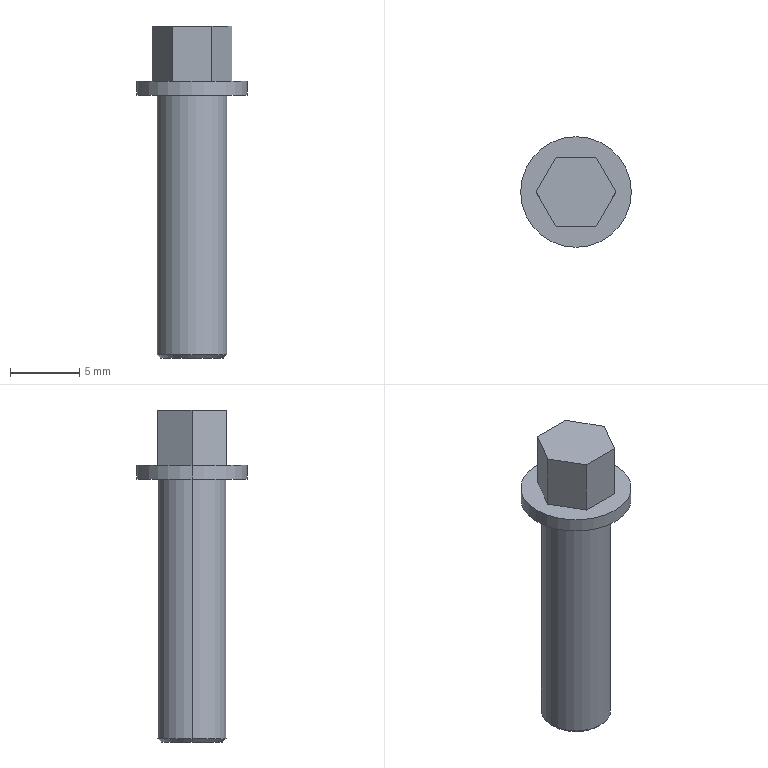Part | SolidWorks | features BaseBody 1 | 1 solid | 16 faces | box 8 x 8 x 24 mm | volume 509.458 mm3 | plane 10 | cylinder 4 | cone 2 | commonest cylinder face diameters 5 x2 8 x2
STEP:
#1=CARTESIAN_POINT('',(2.25,0.,-19.));
#2=VERTEX_POINT('',#1);
#3=CARTESIAN_POINT('',(-2.25,0.,-19.));
#4=VERTEX_POINT('',#3);
#5=CARTESIAN_POINT('',(0.,0.,-19.));
#6=DIRECTION('',(0.,0.,1.));
#7=DIRECTION('',(1.,0.,0.));
#8=AXIS2_PLACEMENT_3D('',#5,#6,#7);
#9=CIRCLE('',#8,2.25);
#10=EDGE_CURVE('',#2,#4,#9,.T.);
#11=ORIENTED_EDGE('',*,*,#10,.T.);
#12=CARTESIAN_POINT('',(-2.5,0.,-18.75));
#13=VERTEX_POINT('',#12);
#14=CARTESIAN_POINT('',(-2.375,0.,-18.875));
#15=DIRECTION('',(-0.7071,0.,0.7071));
#16=VECTOR('',#15,1000.);
#17=LINE('',#14,#16);
#18=EDGE_CURVE('',#4,#13,#17,.T.);
#19=ORIENTED_EDGE('',*,*,#18,.T.);
#20=CARTESIAN_POINT('',(2.5,0.,-18.75));
#21=VERTEX_POINT('',#20);
#22=CARTESIAN_POINT('',(0.,0.,-18.75));
#23=DIRECTION('',(0.,0.,-1.));
#24=DIRECTION('',(1.,0.,0.));
#25=AXIS2_PLACEMENT_3D('',#22,#23,#24);
#26=CIRCLE('',#25,2.5);
#27=EDGE_CURVE('',#13,#21,#26,.T.);
#28=ORIENTED_EDGE('',*,*,#27,.T.);
#29=CARTESIAN_POINT('',(2.375,0.,-18.875));
#30=DIRECTION('',(0.7071,0.,0.7071));
#31=VECTOR('',#30,1000.);
#32=LINE('',#29,#31);
#33=EDGE_CURVE('',#2,#21,#32,.T.);
#34=ORIENTED_EDGE('',*,*,#33,.F.);
#35=EDGE_LOOP('',(#11,#19,#28,#34));
#36=FACE_OUTER_BOUND('',#35,.T.);
#37=CARTESIAN_POINT('',(0.,0.,-18.875));
#38=DIRECTION('',(0.,0.,1.));
#39=DIRECTION('',(1.,0.,0.));
#40=AXIS2_PLACEMENT_3D('',#37,#38,#39);
#41=CONICAL_SURFACE('',#40,2.375,0.7854);
#42=ADVANCED_FACE('',(#36),#41,.T.);
#43=ORIENTED_EDGE('',*,*,#27,.F.);
#44=CARTESIAN_POINT('',(-2.5,0.,0.));
#45=VERTEX_POINT('',#44);
#46=CARTESIAN_POINT('',(-2.5,0.,0.));
#47=DIRECTION('',(0.,0.,1.));
#48=VECTOR('',#47,1000.);
#49=LINE('',#46,#48);
#50=EDGE_CURVE('',#13,#45,#49,.T.);
#51=ORIENTED_EDGE('',*,*,#50,.T.);
#52=CARTESIAN_POINT('',(2.5,0.,0.));
#53=VERTEX_POINT('',#52);
#54=CARTESIAN_POINT('',(0.,0.,0.));
#55=DIRECTION('',(0.,0.,1.));
#56=DIRECTION('',(1.,0.,0.));
#57=AXIS2_PLACEMENT_3D('',#54,#55,#56);
#58=CIRCLE('',#57,2.5);
#59=EDGE_CURVE('',#53,#45,#58,.T.);
#60=ORIENTED_EDGE('',*,*,#59,.F.);
#61=CARTESIAN_POINT('',(2.5,0.,0.));
#62=DIRECTION('',(0.,0.,1.));
#63=VECTOR('',#62,1000.);
#64=LINE('',#61,#63);
#65=EDGE_CURVE('',#21,#53,#64,.T.);
#66=ORIENTED_EDGE('',*,*,#65,.F.);
#67=EDGE_LOOP('',(#43,#51,#60,#66));
#68=FACE_OUTER_BOUND('',#67,.T.);
#69=CARTESIAN_POINT('',(0.,0.,0.));
#70=DIRECTION('',(0.,0.,1.));
#71=DIRECTION('',(1.,0.,0.));
#72=AXIS2_PLACEMENT_3D('',#69,#70,#71);
#73=CYLINDRICAL_SURFACE('',#72,2.5);
#74=ADVANCED_FACE('',(#68),#73,.T.);
#75=CARTESIAN_POINT('',(4.,0.,1.));
#76=VERTEX_POINT('',#75);
#77=CARTESIAN_POINT('',(-4.,0.,1.));
#78=VERTEX_POINT('',#77);
#79=CARTESIAN_POINT('',(0.,0.,1.));
#80=DIRECTION('',(0.,0.,1.));
#81=DIRECTION('',(-1.,0.,0.));
#82=AXIS2_PLACEMENT_3D('',#79,#80,#81);
#83=CIRCLE('',#82,4.);
#84=EDGE_CURVE('',#76,#78,#83,.T.);
#85=ORIENTED_EDGE('',*,*,#84,.F.);
#86=CARTESIAN_POINT('',(4.,0.,0.));
#87=VERTEX_POINT('',#86);
#88=CARTESIAN_POINT('',(4.,0.,0.));
#89=DIRECTION('',(0.,0.,-1.));
#90=VECTOR('',#89,1000.);
#91=LINE('',#88,#90);
#92=EDGE_CURVE('',#76,#87,#91,.T.);
#93=ORIENTED_EDGE('',*,*,#92,.T.);
#94=CARTESIAN_POINT('',(-4.,0.,0.));
#95=VERTEX_POINT('',#94);
#96=CARTESIAN_POINT('',(0.,0.,0.));
#97=DIRECTION('',(0.,0.,-1.));
#98=DIRECTION('',(-1.,0.,0.));
#99=AXIS2_PLACEMENT_3D('',#96,#97,#98);
#100=CIRCLE('',#99,4.);
#101=EDGE_CURVE('',#95,#87,#100,.T.);
#102=ORIENTED_EDGE('',*,*,#101,.F.);
#103=CARTESIAN_POINT('',(-4.,0.,0.));
#104=DIRECTION('',(0.,0.,-1.));
#105=VECTOR('',#104,1000.);
#106=LINE('',#103,#105);
#107=EDGE_CURVE('',#78,#95,#106,.T.);
#108=ORIENTED_EDGE('',*,*,#107,.F.);
#109=EDGE_LOOP('',(#85,#93,#102,#108));
#110=FACE_OUTER_BOUND('',#109,.T.);
#111=CARTESIAN_POINT('',(0.,0.,0.));
#112=DIRECTION('',(0.,0.,-1.));
#113=DIRECTION('',(-1.,0.,0.));
#114=AXIS2_PLACEMENT_3D('',#111,#112,#113);
#115=CYLINDRICAL_SURFACE('',#114,4.);
#116=ADVANCED_FACE('',(#110),#115,.T.);
#117=ORIENTED_EDGE('',*,*,#10,.F.);
#118=CARTESIAN_POINT('',(0.,0.,-19.));
#119=DIRECTION('',(0.,0.,1.));
#120=DIRECTION('',(1.,0.,0.));
#121=AXIS2_PLACEMENT_3D('',#118,#119,#120);
#122=CIRCLE('',#121,2.25);
#123=EDGE_CURVE('',#4,#2,#122,.T.);
#124=ORIENTED_EDGE('',*,*,#123,.F.);
#125=EDGE_LOOP('',(#117,#124));
#126=FACE_OUTER_BOUND('',#125,.T.);
#127=CARTESIAN_POINT('',(0.,0.,-19.));
#128=DIRECTION('',(0.,0.,1.));
#129=DIRECTION('',(1.,0.,0.));
#130=AXIS2_PLACEMENT_3D('',#127,#128,#129);
#131=PLANE('',#130);
#132=ADVANCED_FACE('',(#126),#131,.F.);
#133=CARTESIAN_POINT('',(-1.443,-2.5,1.));
#134=VERTEX_POINT('',#133);
#135=CARTESIAN_POINT('',(-2.887,0.,1.));
#136=VERTEX_POINT('',#135);
#137=CARTESIAN_POINT('',(-2.526,-0.625,1.));
#138=DIRECTION('',(-0.5,0.866,0.));
#139=VECTOR('',#138,1000.);
#140=LINE('',#137,#139);
#141=EDGE_CURVE('',#134,#136,#140,.T.);
#142=ORIENTED_EDGE('',*,*,#141,.F.);
#143=CARTESIAN_POINT('',(-1.443,-2.5,5.));
#144=VERTEX_POINT('',#143);
#145=CARTESIAN_POINT('',(-1.443,-2.5,1.));
#146=DIRECTION('',(0.,0.,1.));
#147=VECTOR('',#146,1000.);
#148=LINE('',#145,#147);
#149=EDGE_CURVE('',#134,#144,#148,.T.);
#150=ORIENTED_EDGE('',*,*,#149,.T.);
#151=CARTESIAN_POINT('',(-2.887,0.,5.));
#152=VERTEX_POINT('',#151);
#153=CARTESIAN_POINT('',(-1.443,-2.5,5.));
#154=DIRECTION('',(0.5,-0.866,0.));
#155=VECTOR('',#154,1000.);
#156=LINE('',#153,#155);
#157=EDGE_CURVE('',#152,#144,#156,.T.);
#158=ORIENTED_EDGE('',*,*,#157,.F.);
#159=CARTESIAN_POINT('',(-2.887,0.,1.));
#160=DIRECTION('',(0.,0.,1.));
#161=VECTOR('',#160,1000.);
#162=LINE('',#159,#161);
#163=EDGE_CURVE('',#136,#152,#162,.T.);
#164=ORIENTED_EDGE('',*,*,#163,.F.);
#165=EDGE_LOOP('',(#142,#150,#158,#164));
#166=FACE_OUTER_BOUND('',#165,.T.);
#167=CARTESIAN_POINT('',(-2.887,0.,1.));
#168=DIRECTION('',(-0.866,-0.5,0.));
#169=DIRECTION('',(-0.5,0.866,0.));
#170=AXIS2_PLACEMENT_3D('',#167,#168,#169);
#171=PLANE('',#170);
#172=ADVANCED_FACE('',(#166),#171,.T.);
#173=CARTESIAN_POINT('',(-1.443,2.5,1.));
#174=VERTEX_POINT('',#173);
#175=CARTESIAN_POINT('',(-1.804,1.875,1.));
#176=DIRECTION('',(0.5,0.866,0.));
#177=VECTOR('',#176,1000.);
#178=LINE('',#175,#177);
#179=EDGE_CURVE('',#136,#174,#178,.T.);
#180=ORIENTED_EDGE('',*,*,#179,.F.);
#181=ORIENTED_EDGE('',*,*,#163,.T.);
#182=CARTESIAN_POINT('',(-1.443,2.5,5.));
#183=VERTEX_POINT('',#182);
#184=CARTESIAN_POINT('',(-2.887,0.,5.));
#185=DIRECTION('',(-0.5,-0.866,0.));
#186=VECTOR('',#185,1000.);
#187=LINE('',#184,#186);
#188=EDGE_CURVE('',#183,#152,#187,.T.);
#189=ORIENTED_EDGE('',*,*,#188,.F.);
#190=CARTESIAN_POINT('',(-1.443,2.5,1.));
#191=DIRECTION('',(0.,0.,1.));
#192=VECTOR('',#191,1000.);
#193=LINE('',#190,#192);
#194=EDGE_CURVE('',#174,#183,#193,.T.);
#195=ORIENTED_EDGE('',*,*,#194,.F.);
#196=EDGE_LOOP('',(#180,#181,#189,#195));
#197=FACE_OUTER_BOUND('',#196,.T.);
#198=CARTESIAN_POINT('',(-1.443,2.5,1.));
#199=DIRECTION('',(-0.866,0.5,0.));
#200=DIRECTION('',(0.,0.,1.));
#201=AXIS2_PLACEMENT_3D('',#198,#199,#200);
#202=PLANE('',#201);
#203=ADVANCED_FACE('',(#197),#202,.T.);
#204=CARTESIAN_POINT('',(1.443,2.5,1.));
#205=VERTEX_POINT('',#204);
#206=CARTESIAN_POINT('',(0.7217,2.5,1.));
#207=DIRECTION('',(1.,0.,0.));
#208=VECTOR('',#207,1000.);
#209=LINE('',#206,#208);
#210=EDGE_CURVE('',#174,#205,#209,.T.);
#211=ORIENTED_EDGE('',*,*,#210,.F.);
#212=ORIENTED_EDGE('',*,*,#194,.T.);
#213=CARTESIAN_POINT('',(1.443,2.5,5.));
#214=VERTEX_POINT('',#213);
#215=CARTESIAN_POINT('',(-1.443,2.5,5.));
#216=DIRECTION('',(-1.,0.,0.));
#217=VECTOR('',#216,1000.);
#218=LINE('',#215,#217);
#219=EDGE_CURVE('',#214,#183,#218,.T.);
#220=ORIENTED_EDGE('',*,*,#219,.F.);
#221=CARTESIAN_POINT('',(1.443,2.5,1.));
#222=DIRECTION('',(0.,0.,1.));
#223=VECTOR('',#222,1000.);
#224=LINE('',#221,#223);
#225=EDGE_CURVE('',#205,#214,#224,.T.);
#226=ORIENTED_EDGE('',*,*,#225,.F.);
#227=EDGE_LOOP('',(#211,#212,#220,#226));
#228=FACE_OUTER_BOUND('',#227,.T.);
#229=CARTESIAN_POINT('',(1.443,2.5,1.));
#230=DIRECTION('',(0.,1.,0.));
#231=DIRECTION('',(1.,0.,0.));
#232=AXIS2_PLACEMENT_3D('',#229,#230,#231);
#233=PLANE('',#232);
#234=ADVANCED_FACE('',(#228),#233,.T.);
#235=CARTESIAN_POINT('',(2.887,0.,1.));
#236=VERTEX_POINT('',#235);
#237=CARTESIAN_POINT('',(2.526,0.625,1.));
#238=DIRECTION('',(0.5,-0.866,0.));
#239=VECTOR('',#238,1000.);
#240=LINE('',#237,#239);
#241=EDGE_CURVE('',#205,#236,#240,.T.);
#242=ORIENTED_EDGE('',*,*,#241,.F.);
#243=ORIENTED_EDGE('',*,*,#225,.T.);
#244=CARTESIAN_POINT('',(2.887,0.,5.));
#245=VERTEX_POINT('',#244);
#246=CARTESIAN_POINT('',(1.443,2.5,5.));
#247=DIRECTION('',(-0.5,0.866,0.));
#248=VECTOR('',#247,1000.);
#249=LINE('',#246,#248);
#250=EDGE_CURVE('',#245,#214,#249,.T.);
#251=ORIENTED_EDGE('',*,*,#250,.F.);
#252=CARTESIAN_POINT('',(2.887,0.,1.));
#253=DIRECTION('',(0.,0.,1.));
#254=VECTOR('',#253,1000.);
#255=LINE('',#252,#254);
#256=EDGE_CURVE('',#236,#245,#255,.T.);
#257=ORIENTED_EDGE('',*,*,#256,.F.);
#258=EDGE_LOOP('',(#242,#243,#251,#257));
#259=FACE_OUTER_BOUND('',#258,.T.);
#260=CARTESIAN_POINT('',(2.887,0.,1.));
#261=DIRECTION('',(0.866,0.5,0.));
#262=DIRECTION('',(0.,0.,-1.));
#263=AXIS2_PLACEMENT_3D('',#260,#261,#262);
#264=PLANE('',#263);
#265=ADVANCED_FACE('',(#259),#264,.T.);
#266=CARTESIAN_POINT('',(1.443,-2.5,1.));
#267=VERTEX_POINT('',#266);
#268=CARTESIAN_POINT('',(1.804,-1.875,1.));
#269=DIRECTION('',(-0.5,-0.866,0.));
#270=VECTOR('',#269,1000.);
#271=LINE('',#268,#270);
#272=EDGE_CURVE('',#236,#267,#271,.T.);
#273=ORIENTED_EDGE('',*,*,#272,.F.);
#274=ORIENTED_EDGE('',*,*,#256,.T.);
#275=CARTESIAN_POINT('',(1.443,-2.5,5.));
#276=VERTEX_POINT('',#275);
#277=CARTESIAN_POINT('',(2.887,0.,5.));
#278=DIRECTION('',(0.5,0.866,0.));
#279=VECTOR('',#278,1000.);
#280=LINE('',#277,#279);
#281=EDGE_CURVE('',#276,#245,#280,.T.);
#282=ORIENTED_EDGE('',*,*,#281,.F.);
#283=CARTESIAN_POINT('',(1.443,-2.5,1.));
#284=DIRECTION('',(0.,0.,1.));
#285=VECTOR('',#284,1000.);
#286=LINE('',#283,#285);
#287=EDGE_CURVE('',#267,#276,#286,.T.);
#288=ORIENTED_EDGE('',*,*,#287,.F.);
#289=EDGE_LOOP('',(#273,#274,#282,#288));
#290=FACE_OUTER_BOUND('',#289,.T.);
#291=CARTESIAN_POINT('',(1.443,-2.5,1.));
#292=DIRECTION('',(0.866,-0.5,0.));
#293=DIRECTION('',(0.,0.,-1.));
#294=AXIS2_PLACEMENT_3D('',#291,#292,#293);
#295=PLANE('',#294);
#296=ADVANCED_FACE('',(#290),#295,.T.);
#297=CARTESIAN_POINT('',(-0.7217,-2.5,1.));
#298=DIRECTION('',(-1.,0.,0.));
#299=VECTOR('',#298,1000.);
#300=LINE('',#297,#299);
#301=EDGE_CURVE('',#267,#134,#300,.T.);
#302=ORIENTED_EDGE('',*,*,#301,.F.);
#303=ORIENTED_EDGE('',*,*,#287,.T.);
#304=CARTESIAN_POINT('',(1.443,-2.5,5.));
#305=DIRECTION('',(1.,0.,0.));
#306=VECTOR('',#305,1000.);
#307=LINE('',#304,#306);
#308=EDGE_CURVE('',#144,#276,#307,.T.);
#309=ORIENTED_EDGE('',*,*,#308,.F.);
#310=ORIENTED_EDGE('',*,*,#149,.F.);
#311=EDGE_LOOP('',(#302,#303,#309,#310));
#312=FACE_OUTER_BOUND('',#311,.T.);
#313=CARTESIAN_POINT('',(-1.443,-2.5,1.));
#314=DIRECTION('',(0.,-1.,0.));
#315=DIRECTION('',(-1.,0.,0.));
#316=AXIS2_PLACEMENT_3D('',#313,#314,#315);
#317=PLANE('',#316);
#318=ADVANCED_FACE('',(#312),#317,.T.);
#319=ORIENTED_EDGE('',*,*,#308,.T.);
#320=ORIENTED_EDGE('',*,*,#281,.T.);
#321=ORIENTED_EDGE('',*,*,#250,.T.);
#322=ORIENTED_EDGE('',*,*,#219,.T.);
#323=ORIENTED_EDGE('',*,*,#188,.T.);
#324=ORIENTED_EDGE('',*,*,#157,.T.);
#325=EDGE_LOOP('',(#319,#320,#321,#322,#323,#324));
#326=FACE_OUTER_BOUND('',#325,.T.);
#327=CARTESIAN_POINT('',(0.,0.,5.));
#328=DIRECTION('',(0.,0.,1.));
#329=DIRECTION('',(1.,0.,0.));
#330=AXIS2_PLACEMENT_3D('',#327,#328,#329);
#331=PLANE('',#330);
#332=ADVANCED_FACE('',(#326),#331,.T.);
#333=ORIENTED_EDGE('',*,*,#59,.T.);
#334=CARTESIAN_POINT('',(0.,0.,0.));
#335=DIRECTION('',(0.,0.,1.));
#336=DIRECTION('',(1.,0.,0.));
#337=AXIS2_PLACEMENT_3D('',#334,#335,#336);
#338=CIRCLE('',#337,2.5);
#339=EDGE_CURVE('',#45,#53,#338,.T.);
#340=ORIENTED_EDGE('',*,*,#339,.T.);
#341=EDGE_LOOP('',(#333,#340));
#342=FACE_BOUND('',#341,.T.);
#343=ORIENTED_EDGE('',*,*,#101,.T.);
#344=CARTESIAN_POINT('',(0.,0.,0.));
#345=DIRECTION('',(0.,0.,-1.));
#346=DIRECTION('',(-1.,0.,0.));
#347=AXIS2_PLACEMENT_3D('',#344,#345,#346);
#348=CIRCLE('',#347,4.);
#349=EDGE_CURVE('',#87,#95,#348,.T.);
#350=ORIENTED_EDGE('',*,*,#349,.T.);
#351=EDGE_LOOP('',(#343,#350));
#352=FACE_OUTER_BOUND('',#351,.T.);
#353=CARTESIAN_POINT('',(0.,0.,0.));
#354=DIRECTION('',(0.,0.,1.));
#355=DIRECTION('',(1.,0.,0.));
#356=AXIS2_PLACEMENT_3D('',#353,#354,#355);
#357=PLANE('',#356);
#358=ADVANCED_FACE('',(#342,#352),#357,.F.);
#359=ORIENTED_EDGE('',*,*,#141,.T.);
#360=ORIENTED_EDGE('',*,*,#179,.T.);
#361=ORIENTED_EDGE('',*,*,#210,.T.);
#362=ORIENTED_EDGE('',*,*,#241,.T.);
#363=ORIENTED_EDGE('',*,*,#272,.T.);
#364=ORIENTED_EDGE('',*,*,#301,.T.);
#365=EDGE_LOOP('',(#359,#360,#361,#362,#363,#364));
#366=FACE_BOUND('',#365,.T.);
#367=CARTESIAN_POINT('',(0.,0.,1.));
#368=DIRECTION('',(0.,0.,1.));
#369=DIRECTION('',(-1.,0.,0.));
#370=AXIS2_PLACEMENT_3D('',#367,#368,#369);
#371=CIRCLE('',#370,4.);
#372=EDGE_CURVE('',#78,#76,#371,.T.);
#373=ORIENTED_EDGE('',*,*,#372,.T.);
#374=ORIENTED_EDGE('',*,*,#84,.T.);
#375=EDGE_LOOP('',(#373,#374));
#376=FACE_OUTER_BOUND('',#375,.T.);
#377=CARTESIAN_POINT('',(0.,0.,1.));
#378=DIRECTION('',(0.,0.,1.));
#379=DIRECTION('',(1.,0.,0.));
#380=AXIS2_PLACEMENT_3D('',#377,#378,#379);
#381=PLANE('',#380);
#382=ADVANCED_FACE('',(#366,#376),#381,.T.);
#383=ORIENTED_EDGE('',*,*,#92,.F.);
#384=ORIENTED_EDGE('',*,*,#372,.F.);
#385=ORIENTED_EDGE('',*,*,#107,.T.);
#386=ORIENTED_EDGE('',*,*,#349,.F.);
#387=EDGE_LOOP('',(#383,#384,#385,#386));
#388=FACE_OUTER_BOUND('',#387,.T.);
#389=CARTESIAN_POINT('',(0.,0.,0.));
#390=DIRECTION('',(0.,0.,-1.));
#391=DIRECTION('',(-1.,0.,0.));
#392=AXIS2_PLACEMENT_3D('',#389,#390,#391);
#393=CYLINDRICAL_SURFACE('',#392,4.);
#394=ADVANCED_FACE('',(#388),#393,.T.);
#395=ORIENTED_EDGE('',*,*,#50,.F.);
#396=CARTESIAN_POINT('',(0.,0.,-18.75));
#397=DIRECTION('',(0.,0.,-1.));
#398=DIRECTION('',(1.,0.,0.));
#399=AXIS2_PLACEMENT_3D('',#396,#397,#398);
#400=CIRCLE('',#399,2.5);
#401=EDGE_CURVE('',#21,#13,#400,.T.);
#402=ORIENTED_EDGE('',*,*,#401,.F.);
#403=ORIENTED_EDGE('',*,*,#65,.T.);
#404=ORIENTED_EDGE('',*,*,#339,.F.);
#405=EDGE_LOOP('',(#395,#402,#403,#404));
#406=FACE_OUTER_BOUND('',#405,.T.);
#407=CARTESIAN_POINT('',(0.,0.,0.));
#408=DIRECTION('',(0.,0.,1.));
#409=DIRECTION('',(1.,0.,0.));
#410=AXIS2_PLACEMENT_3D('',#407,#408,#409);
#411=CYLINDRICAL_SURFACE('',#410,2.5);
#412=ADVANCED_FACE('',(#406),#411,.T.);
#413=ORIENTED_EDGE('',*,*,#18,.F.);
#414=ORIENTED_EDGE('',*,*,#123,.T.);
#415=ORIENTED_EDGE('',*,*,#33,.T.);
#416=ORIENTED_EDGE('',*,*,#401,.T.);
#417=EDGE_LOOP('',(#413,#414,#415,#416));
#418=FACE_OUTER_BOUND('',#417,.T.);
#419=CARTESIAN_POINT('',(0.,0.,-18.875));
#420=DIRECTION('',(0.,0.,1.));
#421=DIRECTION('',(1.,0.,0.));
#422=AXIS2_PLACEMENT_3D('',#419,#420,#421);
#423=CONICAL_SURFACE('',#422,2.375,0.7854);
#424=ADVANCED_FACE('',(#418),#423,.T.);
#425=CLOSED_SHELL('',(#42,#74,#116,#132,#172,#203,#234,#265,#296,#318,#332,#358,#382,#394,#412,#424));
#426=MANIFOLD_SOLID_BREP('',#425);
#427=CARTESIAN_POINT('',(0.,0.,0.));
#428=DIRECTION('',(0.,0.,1.));
#429=DIRECTION('',(1.,0.,0.));
#430=AXIS2_PLACEMENT_3D('',#427,#428,#429);
#431=(LENGTH_UNIT()NAMED_UNIT(*)SI_UNIT(.MILLI.,.METRE.));
#432=UNCERTAINTY_MEASURE_WITH_UNIT(LENGTH_MEASURE(0.00001),#431,'','');
#433=(NAMED_UNIT(*)PLANE_ANGLE_UNIT()SI_UNIT($,.RADIAN.));
#434=(NAMED_UNIT(*)SI_UNIT($,.STERADIAN.)SOLID_ANGLE_UNIT());
#435=(GEOMETRIC_REPRESENTATION_CONTEXT(3)GLOBAL_UNCERTAINTY_ASSIGNED_CONTEXT((#432))GLOBAL_UNIT_ASSIGNED_CONTEXT((#431,#433,#434))REPRESENTATION_CONTEXT('',''));
#436=ADVANCED_BREP_SHAPE_REPRESENTATION('',(#426,#430),#435);